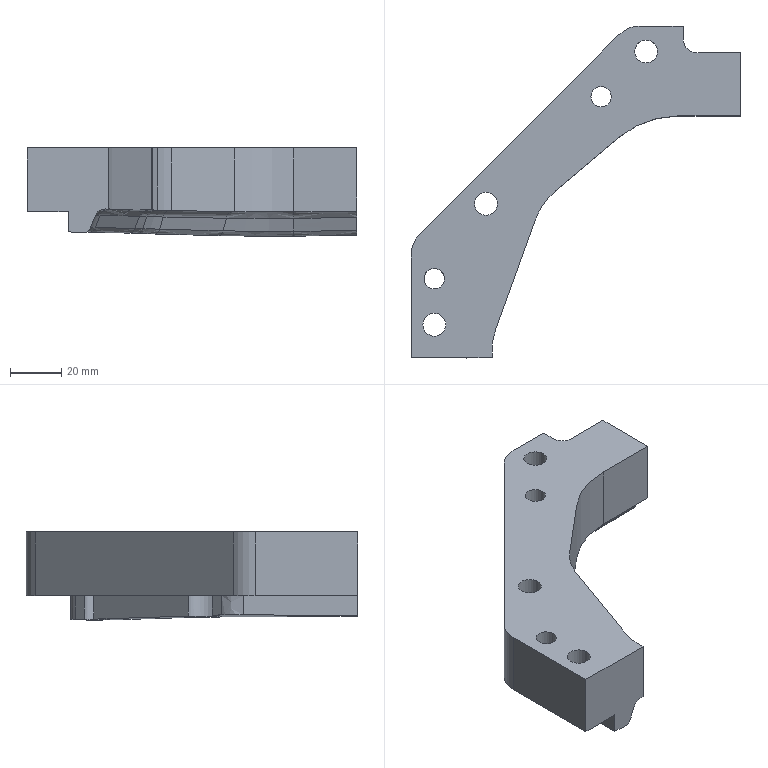Part | STEP file | 809_id1594_x_t | 1 solid | 72 faces | box 129 x 130 x 34.601 mm | volume 147942 mm3 | spline 39 | plane 19 | cylinder 14 | commonest cylinder face diameters 9 x3 10 x3 14 x3 8 x2 24 x2 12 x1